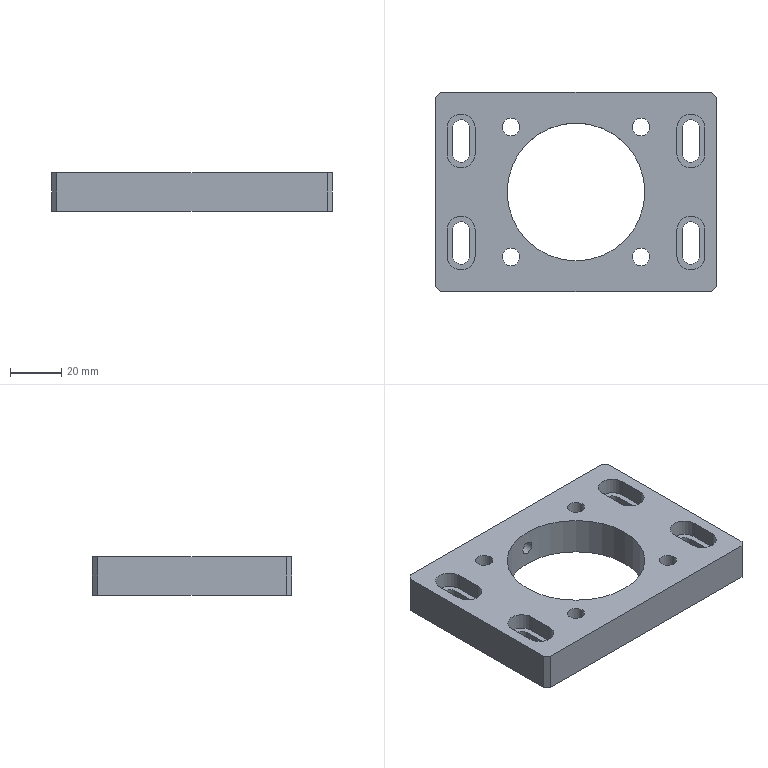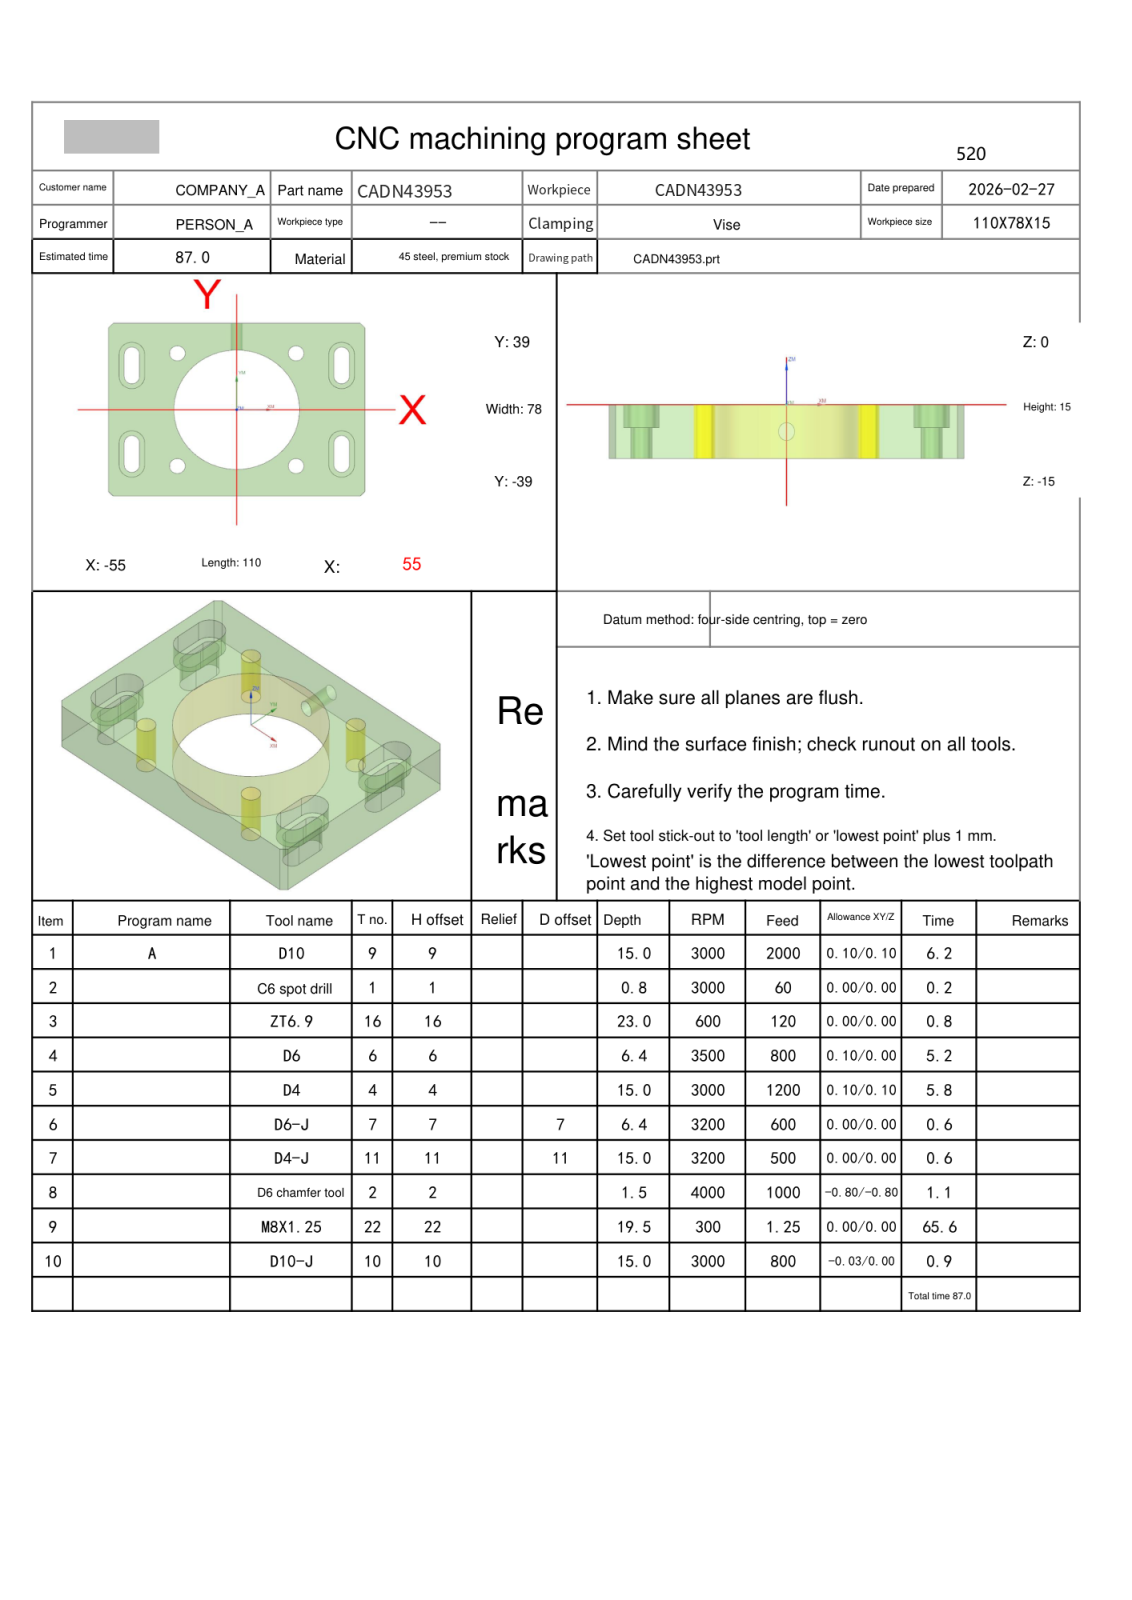NC program | NX | posted by the shop | part box 110 x 78 x 15 mm
Lines 2258 to 4088 of 4469, first 1188 of 1831 lines:
N5 T04 M06
(D4  D=4. R=0. H=04 ce=0.10 di=0.10)
G00 G90 G54 X-46.2 Y-20. M03 S3000
G43 H04 Z50.
M08
Z-5.9
G01 Y-25. Z-5.927 F1200.
G03 X-45. Y-26.2 Z-5.937 I1.2 J0.0
X-43.8 Y-25. Z-5.948 I0.0 J1.2
G01 Y-15. Z-6.002
G03 X-45. Y-13.8 Z-6.012 I-1.2 J0.0
X-46.2 Y-15. Z-6.022 I0.0 J-1.2
G01 Y-25. Z-6.076
G03 X-45. Y-26.2 Z-6.086 I1.2 J0.0
X-43.8 Y-25. Z-6.097 I0.0 J1.2
G01 Y-15. Z-6.151
G03 X-45. Y-13.8 Z-6.161 I-1.2 J0.0
X-46.2 Y-15. Z-6.171 I0.0 J-1.2
G01 Y-25. Z-6.225
G03 X-45. Y-26.2 Z-6.236 I1.2 J0.0
X-43.8 Y-25. Z-6.246 I0.0 J1.2
G01 Y-15. Z-6.3
G03 X-45. Y-13.8 Z-6.31 I-1.2 J0.0
X-46.2 Y-15. Z-6.32 I0.0 J-1.2
G01 Y-25. Z-6.375
G03 X-45. Y-26.2 Z-6.385 I1.2 J0.0
X-43.8 Y-25. Z-6.395 I0.0 J1.2
G01 Y-15. Z-6.449
G03 X-45. Y-13.8 Z-6.459 I-1.2 J0.0
X-46.2 Y-15. Z-6.47 I0.0 J-1.2
G01 Y-25. Z-6.524
G03 X-45. Y-26.2 Z-6.534 I1.2 J0.0
X-43.8 Y-25. Z-6.544 I0.0 J1.2
G01 Y-15. Z-6.598
G03 X-45. Y-13.8 Z-6.609 I-1.2 J0.0
X-46.2 Y-15. Z-6.619 I0.0 J-1.2
G01 Y-25. Z-6.673
G03 X-45. Y-26.2 Z-6.683 I1.2 J0.0
X-43.8 Y-25. Z-6.693 I0.0 J1.2
G01 Y-15. Z-6.748
G03 X-45. Y-13.8 Z-6.758 I-1.2 J0.0
X-46.2 Y-15. Z-6.768 I0.0 J-1.2
G01 Y-25. Z-6.822
G03 X-45. Y-26.2 Z-6.832 I1.2 J0.0
X-43.8 Y-25. Z-6.843 I0.0 J1.2
G01 Y-15. Z-6.897
G03 X-45. Y-13.8 Z-6.907 I-1.2 J0.0
X-46.2 Y-15. Z-6.917 I0.0 J-1.2
G01 Y-25. Z-6.971
G03 X-45. Y-26.2 Z-6.982 I1.2 J0.0
X-43.8 Y-25. Z-6.992 I0.0 J1.2
G01 Y-15. Z-7.046
G03 X-45. Y-13.8 Z-7.056 I-1.2 J0.0
X-46.2 Y-15. Z-7.066 I0.0 J-1.2
G01 Y-25. Z-7.121
G03 X-45. Y-26.2 Z-7.131 I1.2 J0.0
X-43.8 Y-25. Z-7.141 I0.0 J1.2
G01 Y-15. Z-7.195
G03 X-45. Y-13.8 Z-7.205 I-1.2 J0.0
X-46.2 Y-15. Z-7.216 I0.0 J-1.2
G01 Y-25. Z-7.27
G03 X-45. Y-26.2 Z-7.28 I1.2 J0.0
X-43.8 Y-25. Z-7.29 I0.0 J1.2
G01 Y-15. Z-7.344
G03 X-45. Y-13.8 Z-7.355 I-1.2 J0.0
X-46.2 Y-15. Z-7.365 I0.0 J-1.2
G01 Y-25. Z-7.419
G03 X-45. Y-26.2 Z-7.429 I1.2 J0.0
X-43.8 Y-25. Z-7.439 I0.0 J1.2
G01 Y-15. Z-7.493
G03 X-45. Y-13.8 Z-7.504 I-1.2 J0.0
X-46.2 Y-15. Z-7.514 I0.0 J-1.2
G01 Y-25. Z-7.568
G03 X-45. Y-26.2 Z-7.578 I1.2 J0.0
X-43.8 Y-25. Z-7.588 I0.0 J1.2
G01 Y-15. Z-7.643
G03 X-45. Y-13.8 Z-7.653 I-1.2 J0.0
X-46.2 Y-15. Z-7.663 I0.0 J-1.2
G01 Y-25. Z-7.717
G03 X-45. Y-26.2 Z-7.727 I1.2 J0.0
X-43.8 Y-25. Z-7.738 I0.0 J1.2
G01 Y-15. Z-7.792
G03 X-45. Y-13.8 Z-7.802 I-1.2 J0.0
X-46.2 Y-15. Z-7.812 I0.0 J-1.2
G01 Y-25. Z-7.866
G03 X-45. Y-26.2 Z-7.877 I1.2 J0.0
X-43.8 Y-25. Z-7.887 I0.0 J1.2
G01 Y-15. Z-7.941
G03 X-45. Y-13.8 Z-7.951 I-1.2 J0.0
X-46.2 Y-15. Z-7.961 I0.0 J-1.2
G01 Y-25. Z-8.016
G03 X-45. Y-26.2 Z-8.026 I1.2 J0.0
X-43.8 Y-25. Z-8.036 I0.0 J1.2
G01 Y-15. Z-8.09
G03 X-45. Y-13.8 Z-8.1 I-1.2 J0.0
X-46.2 Y-15. Z-8.111 I0.0 J-1.2
G01 Y-25. Z-8.165
G03 X-45. Y-26.2 Z-8.175 I1.2 J0.0
X-43.8 Y-25. Z-8.185 I0.0 J1.2
G01 Y-15. Z-8.239
G03 X-45. Y-13.8 Z-8.25 I-1.2 J0.0
X-46.2 Y-15. Z-8.26 I0.0 J-1.2
G01 Y-25. Z-8.314
G03 X-45. Y-26.2 Z-8.324 I1.2 J0.0
X-43.8 Y-25. Z-8.334 I0.0 J1.2
G01 Y-15. Z-8.389
G03 X-45. Y-13.8 Z-8.399 I-1.2 J0.0
X-46.2 Y-15. Z-8.409 I0.0 J-1.2
G01 Y-25. Z-8.463
G03 X-45. Y-26.2 Z-8.473 I1.2 J0.0
X-43.8 Y-25. Z-8.484 I0.0 J1.2
G01 Y-15. Z-8.538
G03 X-45. Y-13.8 Z-8.548 I-1.2 J0.0
X-46.2 Y-15. Z-8.558 I0.0 J-1.2
G01 Y-25. Z-8.612
G03 X-45. Y-26.2 Z-8.623 I1.2 J0.0
X-43.8 Y-25. Z-8.633 I0.0 J1.2
G01 Y-15. Z-8.687
G03 X-45. Y-13.8 Z-8.697 I-1.2 J0.0
X-46.2 Y-15. Z-8.707 I0.0 J-1.2
G01 Y-25. Z-8.762
G03 X-45. Y-26.2 Z-8.772 I1.2 J0.0
X-43.8 Y-25. Z-8.782 I0.0 J1.2
G01 Y-15. Z-8.836
G03 X-45. Y-13.8 Z-8.846 I-1.2 J0.0
X-46.2 Y-15. Z-8.857 I0.0 J-1.2
G01 Y-25. Z-8.911
G03 X-45. Y-26.2 Z-8.921 I1.2 J0.0
X-43.8 Y-25. Z-8.931 I0.0 J1.2
G01 Y-15. Z-8.985
G03 X-45. Y-13.8 Z-8.995 I-1.2 J0.0
X-46.2 Y-15. Z-9.006 I0.0 J-1.2
G01 Y-25. Z-9.06
G03 X-45. Y-26.2 Z-9.07 I1.2 J0.0
X-43.8 Y-25. Z-9.08 I0.0 J1.2
G01 Y-15. Z-9.134
G03 X-45. Y-13.8 Z-9.145 I-1.2 J0.0
X-46.2 Y-15. Z-9.155 I0.0 J-1.2
G01 Y-25. Z-9.209
G03 X-45. Y-26.2 Z-9.219 I1.2 J0.0
X-43.8 Y-25. Z-9.229 I0.0 J1.2
G01 Y-15. Z-9.284
G03 X-45. Y-13.8 Z-9.294 I-1.2 J0.0
X-46.2 Y-15. Z-9.304 I0.0 J-1.2
G01 Y-25. Z-9.358
G03 X-45. Y-26.2 Z-9.368 I1.2 J0.0
X-43.8 Y-25. Z-9.379 I0.0 J1.2
G01 Y-15. Z-9.433
G03 X-45. Y-13.8 Z-9.443 I-1.2 J0.0
X-46.2 Y-15. Z-9.453 I0.0 J-1.2
G01 Y-25. Z-9.507
G03 X-45. Y-26.2 Z-9.518 I1.2 J0.0
X-43.8 Y-25. Z-9.528 I0.0 J1.2
G01 Y-15. Z-9.582
G03 X-45. Y-13.8 Z-9.592 I-1.2 J0.0
X-46.2 Y-15. Z-9.602 I0.0 J-1.2
G01 Y-25. Z-9.657
G03 X-45. Y-26.2 Z-9.667 I1.2 J0.0
X-43.8 Y-25. Z-9.677 I0.0 J1.2
G01 Y-15. Z-9.731
G03 X-45. Y-13.8 Z-9.741 I-1.2 J0.0
X-46.2 Y-15. Z-9.752 I0.0 J-1.2
G01 Y-25. Z-9.806
G03 X-45. Y-26.2 Z-9.816 I1.2 J0.0
X-43.8 Y-25. Z-9.826 I0.0 J1.2
G01 Y-15. Z-9.88
G03 X-45. Y-13.8 Z-9.891 I-1.2 J0.0
X-46.2 Y-15. Z-9.901 I0.0 J-1.2
G01 Y-25. Z-9.955
G03 X-45. Y-26.2 Z-9.965 I1.2 J0.0
X-43.8 Y-25. Z-9.975 I0.0 J1.2
G01 Y-15. Z-10.03
G03 X-45. Y-13.8 Z-10.04 I-1.2 J0.0
X-46.2 Y-15. Z-10.05 I0.0 J-1.2
G01 Y-25. Z-10.104
G03 X-45. Y-26.2 Z-10.114 I1.2 J0.0
X-43.8 Y-25. Z-10.125 I0.0 J1.2
G01 Y-15. Z-10.179
G03 X-45. Y-13.8 Z-10.189 I-1.2 J0.0
X-46.2 Y-15. Z-10.199 I0.0 J-1.2
G01 Y-25. Z-10.253
G03 X-45. Y-26.2 Z-10.264 I1.2 J0.0
X-43.8 Y-25. Z-10.274 I0.0 J1.2
G01 Y-15. Z-10.328
G03 X-45. Y-13.8 Z-10.338 I-1.2 J0.0
X-46.2 Y-15. Z-10.348 I0.0 J-1.2
G01 Y-25. Z-10.402
G03 X-45. Y-26.2 Z-10.413 I1.2 J0.0
X-43.8 Y-25. Z-10.423 I0.0 J1.2
G01 Y-15. Z-10.477
G03 X-45. Y-13.8 Z-10.487 I-1.2 J0.0
X-46.2 Y-15. Z-10.498 I0.0 J-1.2
G01 Y-25. Z-10.552
G03 X-45. Y-26.2 Z-10.562 I1.2 J0.0
X-43.8 Y-25. Z-10.572 I0.0 J1.2
G01 Y-15. Z-10.626
G03 X-45. Y-13.8 Z-10.636 I-1.2 J0.0
X-46.2 Y-15. Z-10.647 I0.0 J-1.2
G01 Y-25. Z-10.701
G03 X-45. Y-26.2 Z-10.711 I1.2 J0.0
X-43.8 Y-25. Z-10.721 I0.0 J1.2
G01 Y-15. Z-10.775
G03 X-45. Y-13.8 Z-10.786 I-1.2 J0.0
X-46.2 Y-15. Z-10.796 I0.0 J-1.2
G01 Y-25. Z-10.85
G03 X-45. Y-26.2 Z-10.86 I1.2 J0.0
X-43.8 Y-25. Z-10.87 I0.0 J1.2
G01 Y-15. Z-10.925
G03 X-45. Y-13.8 Z-10.935 I-1.2 J0.0
X-46.2 Y-15. Z-10.945 I0.0 J-1.2
G01 Y-25. Z-10.999
G03 X-45. Y-26.2 Z-11.009 I1.2 J0.0
X-43.8 Y-25. Z-11.02 I0.0 J1.2
G01 Y-15. Z-11.074
G03 X-45. Y-13.8 Z-11.084 I-1.2 J0.0
X-46.2 Y-15. Z-11.094 I0.0 J-1.2
G01 Y-25. Z-11.148
G03 X-45. Y-26.2 Z-11.159 I1.2 J0.0
X-43.8 Y-25. Z-11.169 I0.0 J1.2
G01 Y-15. Z-11.223
G03 X-45. Y-13.8 Z-11.233 I-1.2 J0.0
X-46.2 Y-15. Z-11.243 I0.0 J-1.2
G01 Y-25. Z-11.298
G03 X-45. Y-26.2 Z-11.308 I1.2 J0.0
X-43.8 Y-25. Z-11.318 I0.0 J1.2
G01 Y-15. Z-11.372
G03 X-45. Y-13.8 Z-11.382 I-1.2 J0.0
X-46.2 Y-15. Z-11.393 I0.0 J-1.2
G01 Y-25. Z-11.447
G03 X-45. Y-26.2 Z-11.457 I1.2 J0.0
X-43.8 Y-25. Z-11.467 I0.0 J1.2
G01 Y-15. Z-11.521
G03 X-45. Y-13.8 Z-11.532 I-1.2 J0.0
X-46.2 Y-15. Z-11.542 I0.0 J-1.2
G01 Y-25. Z-11.596
G03 X-45. Y-26.2 Z-11.606 I1.2 J0.0
X-43.8 Y-25. Z-11.616 I0.0 J1.2
G01 Y-15. Z-11.671
G03 X-45. Y-13.8 Z-11.681 I-1.2 J0.0
X-46.2 Y-15. Z-11.691 I0.0 J-1.2
G01 Y-25. Z-11.745
G03 X-45. Y-26.2 Z-11.755 I1.2 J0.0
X-43.8 Y-25. Z-11.766 I0.0 J1.2
G01 Y-15. Z-11.82
G03 X-45. Y-13.8 Z-11.83 I-1.2 J0.0
X-46.2 Y-15. Z-11.84 I0.0 J-1.2
G01 Y-25. Z-11.894
G03 X-45. Y-26.2 Z-11.905 I1.2 J0.0
X-43.8 Y-25. Z-11.915 I0.0 J1.2
G01 Y-15. Z-11.969
G03 X-45. Y-13.8 Z-11.979 I-1.2 J0.0
X-46.2 Y-15. Z-11.989 I0.0 J-1.2
G01 Y-25. Z-12.043
G03 X-45. Y-26.2 Z-12.054 I1.2 J0.0
X-43.8 Y-25. Z-12.064 I0.0 J1.2
G01 Y-15. Z-12.118
G03 X-45. Y-13.8 Z-12.128 I-1.2 J0.0
X-46.2 Y-15. Z-12.138 I0.0 J-1.2
G01 Y-25. Z-12.193
G03 X-45. Y-26.2 Z-12.203 I1.2 J0.0
X-43.8 Y-25. Z-12.213 I0.0 J1.2
G01 Y-15. Z-12.267
G03 X-45. Y-13.8 Z-12.277 I-1.2 J0.0
X-46.2 Y-15. Z-12.288 I0.0 J-1.2
G01 Y-25. Z-12.342
G03 X-45. Y-26.2 Z-12.352 I1.2 J0.0
X-43.8 Y-25. Z-12.362 I0.0 J1.2
G01 Y-15. Z-12.416
G03 X-45. Y-13.8 Z-12.427 I-1.2 J0.0
X-46.2 Y-15. Z-12.437 I0.0 J-1.2
G01 Y-25. Z-12.491
G03 X-45. Y-26.2 Z-12.501 I1.2 J0.0
X-43.8 Y-25. Z-12.511 I0.0 J1.2
G01 Y-15. Z-12.566
G03 X-45. Y-13.8 Z-12.576 I-1.2 J0.0
X-46.2 Y-15. Z-12.586 I0.0 J-1.2
G01 Y-25. Z-12.64
G03 X-45. Y-26.2 Z-12.65 I1.2 J0.0
X-43.8 Y-25. Z-12.661 I0.0 J1.2
G01 Y-15. Z-12.715
G03 X-45. Y-13.8 Z-12.725 I-1.2 J0.0
X-46.2 Y-15. Z-12.735 I0.0 J-1.2
G01 Y-25. Z-12.789
G03 X-45. Y-26.2 Z-12.8 I1.2 J0.0
X-43.8 Y-25. Z-12.81 I0.0 J1.2
G01 Y-15. Z-12.864
G03 X-45. Y-13.8 Z-12.874 I-1.2 J0.0
X-46.2 Y-15. Z-12.884 I0.0 J-1.2
G01 Y-25. Z-12.939
G03 X-45. Y-26.2 Z-12.949 I1.2 J0.0
X-43.8 Y-25. Z-12.959 I0.0 J1.2
G01 Y-15. Z-13.013
G03 X-45. Y-13.8 Z-13.023 I-1.2 J0.0
X-46.2 Y-15. Z-13.034 I0.0 J-1.2
G01 Y-25. Z-13.088
G03 X-45. Y-26.2 Z-13.098 I1.2 J0.0
X-43.8 Y-25. Z-13.108 I0.0 J1.2
G01 Y-15. Z-13.162
G03 X-45. Y-13.8 Z-13.173 I-1.2 J0.0
X-46.2 Y-15. Z-13.183 I0.0 J-1.2
G01 Y-25. Z-13.237
G03 X-45. Y-26.2 Z-13.247 I1.2 J0.0
X-43.8 Y-25. Z-13.257 I0.0 J1.2
G01 Y-15. Z-13.312
G03 X-45. Y-13.8 Z-13.322 I-1.2 J0.0
X-46.2 Y-15. Z-13.332 I0.0 J-1.2
G01 Y-25. Z-13.386
G03 X-45. Y-26.2 Z-13.396 I1.2 J0.0
X-43.8 Y-25. Z-13.407 I0.0 J1.2
G01 Y-15. Z-13.461
G03 X-45. Y-13.8 Z-13.471 I-1.2 J0.0
X-46.2 Y-15. Z-13.481 I0.0 J-1.2
G01 Y-25. Z-13.535
G03 X-45. Y-26.2 Z-13.545 I1.2 J0.0
X-43.8 Y-25. Z-13.556 I0.0 J1.2
G01 Y-15. Z-13.61
G03 X-45. Y-13.8 Z-13.62 I-1.2 J0.0
X-46.2 Y-15. Z-13.63 I0.0 J-1.2
G01 Y-25. Z-13.684
G03 X-45. Y-26.2 Z-13.695 I1.2 J0.0
X-43.8 Y-25. Z-13.705 I0.0 J1.2
G01 Y-15. Z-13.759
G03 X-45. Y-13.8 Z-13.769 I-1.2 J0.0
X-46.2 Y-15. Z-13.779 I0.0 J-1.2
G01 Y-25. Z-13.834
G03 X-45. Y-26.2 Z-13.844 I1.2 J0.0
X-43.8 Y-25. Z-13.854 I0.0 J1.2
G01 Y-15. Z-13.908
G03 X-45. Y-13.8 Z-13.918 I-1.2 J0.0
X-46.2 Y-15. Z-13.929 I0.0 J-1.2
G01 Y-25. Z-13.983
G03 X-45. Y-26.2 Z-13.993 I1.2 J0.0
X-43.8 Y-25. Z-14.003 I0.0 J1.2
G01 Y-15. Z-14.057
G03 X-45. Y-13.8 Z-14.068 I-1.2 J0.0
X-46.2 Y-15. Z-14.078 I0.0 J-1.2
G01 Y-25. Z-14.132
G03 X-45. Y-26.2 Z-14.142 I1.2 J0.0
X-43.8 Y-25. Z-14.152 I0.0 J1.2
G01 Y-15. Z-14.207
G03 X-45. Y-13.8 Z-14.217 I-1.2 J0.0
X-46.2 Y-15. Z-14.227 I0.0 J-1.2
G01 Y-25. Z-14.281
G03 X-45. Y-26.2 Z-14.291 I1.2 J0.0
X-43.8 Y-25. Z-14.302 I0.0 J1.2
G01 Y-15. Z-14.356
G03 X-45. Y-13.8 Z-14.366 I-1.2 J0.0
X-46.2 Y-15. Z-14.376 I0.0 J-1.2
G01 Y-25. Z-14.43
G03 X-45. Y-26.2 Z-14.441 I1.2 J0.0
X-43.8 Y-25. Z-14.451 I0.0 J1.2
G01 Y-15. Z-14.505
G03 X-45. Y-13.8 Z-14.515 I-1.2 J0.0
X-46.2 Y-15. Z-14.525 I0.0 J-1.2
G01 Y-25. Z-14.58
G03 X-45. Y-26.2 Z-14.59 I1.2 J0.0
X-43.8 Y-25. Z-14.6 I0.0 J1.2
G01 Y-15. Z-14.654
G03 X-45. Y-13.8 Z-14.664 I-1.2 J0.0
X-46.2 Y-15. Z-14.675 I0.0 J-1.2
G01 Y-25. Z-14.729
G03 X-45. Y-26.2 Z-14.739 I1.2 J0.0
X-43.8 Y-25. Z-14.749 I0.0 J1.2
G01 Y-15. Z-14.803
G03 X-45. Y-13.8 Z-14.814 I-1.2 J0.0
X-46.2 Y-15. Z-14.824 I0.0 J-1.2
G01 Y-25. Z-14.878
G03 X-45. Y-26.2 Z-14.888 I1.2 J0.0
X-43.8 Y-25. Z-14.898 I0.0 J1.2
G01 Y-15. Z-14.952
G03 X-45. Y-13.8 Z-14.963 I-1.2 J0.0
X-46.2 Y-15. Z-14.973 I0.0 J-1.2
G01 Y-20. Z-15.
Y-25.
G03 X-45. Y-26.2 I1.2 J0.0
X-43.8 Y-25. I0.0 J1.2
G01 Y-15.
G03 X-45. Y-13.8 I-1.2 J0.0
X-46.2 Y-15. I0.0 J-1.2
G01 Y-20.
Y-20.5
Z-14.
G00 Z50.
Y20.
Z-5.9
G01 Y15. Z-5.927
G03 X-45. Y13.8 Z-5.937 I1.2 J0.0
X-43.8 Y15. Z-5.948 I0.0 J1.2
G01 Y25. Z-6.002
G03 X-45. Y26.2 Z-6.012 I-1.2 J0.0
X-46.2 Y25. Z-6.022 I0.0 J-1.2
G01 Y15. Z-6.076
G03 X-45. Y13.8 Z-6.086 I1.2 J0.0
X-43.8 Y15. Z-6.097 I0.0 J1.2
G01 Y25. Z-6.151
G03 X-45. Y26.2 Z-6.161 I-1.2 J0.0
X-46.2 Y25. Z-6.171 I0.0 J-1.2
G01 Y15. Z-6.225
G03 X-45. Y13.8 Z-6.236 I1.2 J0.0
X-43.8 Y15. Z-6.246 I0.0 J1.2
G01 Y25. Z-6.3
G03 X-45. Y26.2 Z-6.31 I-1.2 J0.0
X-46.2 Y25. Z-6.32 I0.0 J-1.2
G01 Y15. Z-6.375
G03 X-45. Y13.8 Z-6.385 I1.2 J0.0
X-43.8 Y15. Z-6.395 I0.0 J1.2
G01 Y25. Z-6.449
G03 X-45. Y26.2 Z-6.459 I-1.2 J0.0
X-46.2 Y25. Z-6.47 I0.0 J-1.2
G01 Y15. Z-6.524
G03 X-45. Y13.8 Z-6.534 I1.2 J0.0
X-43.8 Y15. Z-6.544 I0.0 J1.2
G01 Y25. Z-6.598
G03 X-45. Y26.2 Z-6.609 I-1.2 J0.0
X-46.2 Y25. Z-6.619 I0.0 J-1.2
G01 Y15. Z-6.673
G03 X-45. Y13.8 Z-6.683 I1.2 J0.0
X-43.8 Y15. Z-6.693 I0.0 J1.2
G01 Y25. Z-6.748
G03 X-45. Y26.2 Z-6.758 I-1.2 J0.0
X-46.2 Y25. Z-6.768 I0.0 J-1.2
G01 Y15. Z-6.822
G03 X-45. Y13.8 Z-6.832 I1.2 J0.0
X-43.8 Y15. Z-6.843 I0.0 J1.2
G01 Y25. Z-6.897
G03 X-45. Y26.2 Z-6.907 I-1.2 J0.0
X-46.2 Y25. Z-6.917 I0.0 J-1.2
G01 Y15. Z-6.971
G03 X-45. Y13.8 Z-6.982 I1.2 J0.0
X-43.8 Y15. Z-6.992 I0.0 J1.2
G01 Y25. Z-7.046
G03 X-45. Y26.2 Z-7.056 I-1.2 J0.0
X-46.2 Y25. Z-7.066 I0.0 J-1.2
G01 Y15. Z-7.121
G03 X-45. Y13.8 Z-7.131 I1.2 J0.0
X-43.8 Y15. Z-7.141 I0.0 J1.2
G01 Y25. Z-7.195
G03 X-45. Y26.2 Z-7.205 I-1.2 J0.0
X-46.2 Y25. Z-7.216 I0.0 J-1.2
G01 Y15. Z-7.27
G03 X-45. Y13.8 Z-7.28 I1.2 J0.0
X-43.8 Y15. Z-7.29 I0.0 J1.2
G01 Y25. Z-7.344
G03 X-45. Y26.2 Z-7.355 I-1.2 J0.0
X-46.2 Y25. Z-7.365 I0.0 J-1.2
G01 Y15. Z-7.419
G03 X-45. Y13.8 Z-7.429 I1.2 J0.0
X-43.8 Y15. Z-7.439 I0.0 J1.2
G01 Y25. Z-7.493
G03 X-45. Y26.2 Z-7.504 I-1.2 J0.0
X-46.2 Y25. Z-7.514 I0.0 J-1.2
G01 Y15. Z-7.568
G03 X-45. Y13.8 Z-7.578 I1.2 J0.0
X-43.8 Y15. Z-7.588 I0.0 J1.2
G01 Y25. Z-7.643
G03 X-45. Y26.2 Z-7.653 I-1.2 J0.0
X-46.2 Y25. Z-7.663 I0.0 J-1.2
G01 Y15. Z-7.717
G03 X-45. Y13.8 Z-7.727 I1.2 J0.0
X-43.8 Y15. Z-7.738 I0.0 J1.2
G01 Y25. Z-7.792
G03 X-45. Y26.2 Z-7.802 I-1.2 J0.0
X-46.2 Y25. Z-7.812 I0.0 J-1.2
G01 Y15. Z-7.866
G03 X-45. Y13.8 Z-7.877 I1.2 J0.0
X-43.8 Y15. Z-7.887 I0.0 J1.2
G01 Y25. Z-7.941
G03 X-45. Y26.2 Z-7.951 I-1.2 J0.0
X-46.2 Y25. Z-7.961 I0.0 J-1.2
G01 Y15. Z-8.016
G03 X-45. Y13.8 Z-8.026 I1.2 J0.0
X-43.8 Y15. Z-8.036 I0.0 J1.2
G01 Y25. Z-8.09
G03 X-45. Y26.2 Z-8.1 I-1.2 J0.0
X-46.2 Y25. Z-8.111 I0.0 J-1.2
G01 Y15. Z-8.165
G03 X-45. Y13.8 Z-8.175 I1.2 J0.0
X-43.8 Y15. Z-8.185 I0.0 J1.2
G01 Y25. Z-8.239
G03 X-45. Y26.2 Z-8.25 I-1.2 J0.0
X-46.2 Y25. Z-8.26 I0.0 J-1.2
G01 Y15. Z-8.314
G03 X-45. Y13.8 Z-8.324 I1.2 J0.0
X-43.8 Y15. Z-8.334 I0.0 J1.2
G01 Y25. Z-8.389
G03 X-45. Y26.2 Z-8.399 I-1.2 J0.0
X-46.2 Y25. Z-8.409 I0.0 J-1.2
G01 Y15. Z-8.463
G03 X-45. Y13.8 Z-8.473 I1.2 J0.0
X-43.8 Y15. Z-8.484 I0.0 J1.2
G01 Y25. Z-8.538
G03 X-45. Y26.2 Z-8.548 I-1.2 J0.0
X-46.2 Y25. Z-8.558 I0.0 J-1.2
G01 Y15. Z-8.612
G03 X-45. Y13.8 Z-8.623 I1.2 J0.0
X-43.8 Y15. Z-8.633 I0.0 J1.2
G01 Y25. Z-8.687
G03 X-45. Y26.2 Z-8.697 I-1.2 J0.0
X-46.2 Y25. Z-8.707 I0.0 J-1.2
G01 Y15. Z-8.762
G03 X-45. Y13.8 Z-8.772 I1.2 J0.0
X-43.8 Y15. Z-8.782 I0.0 J1.2
G01 Y25. Z-8.836
G03 X-45. Y26.2 Z-8.846 I-1.2 J0.0
X-46.2 Y25. Z-8.857 I0.0 J-1.2
G01 Y15. Z-8.911
G03 X-45. Y13.8 Z-8.921 I1.2 J0.0
X-43.8 Y15. Z-8.931 I0.0 J1.2
G01 Y25. Z-8.985
G03 X-45. Y26.2 Z-8.995 I-1.2 J0.0
X-46.2 Y25. Z-9.006 I0.0 J-1.2
G01 Y15. Z-9.06
G03 X-45. Y13.8 Z-9.07 I1.2 J0.0
X-43.8 Y15. Z-9.08 I0.0 J1.2
G01 Y25. Z-9.134
G03 X-45. Y26.2 Z-9.145 I-1.2 J0.0
X-46.2 Y25. Z-9.155 I0.0 J-1.2
G01 Y15. Z-9.209
G03 X-45. Y13.8 Z-9.219 I1.2 J0.0
X-43.8 Y15. Z-9.229 I0.0 J1.2
G01 Y25. Z-9.284
G03 X-45. Y26.2 Z-9.294 I-1.2 J0.0
X-46.2 Y25. Z-9.304 I0.0 J-1.2
G01 Y15. Z-9.358
G03 X-45. Y13.8 Z-9.368 I1.2 J0.0
X-43.8 Y15. Z-9.379 I0.0 J1.2
G01 Y25. Z-9.433
G03 X-45. Y26.2 Z-9.443 I-1.2 J0.0
X-46.2 Y25. Z-9.453 I0.0 J-1.2
G01 Y15. Z-9.507
G03 X-45. Y13.8 Z-9.518 I1.2 J0.0
X-43.8 Y15. Z-9.528 I0.0 J1.2
G01 Y25. Z-9.582
G03 X-45. Y26.2 Z-9.592 I-1.2 J0.0
X-46.2 Y25. Z-9.602 I0.0 J-1.2
G01 Y15. Z-9.657
G03 X-45. Y13.8 Z-9.667 I1.2 J0.0
X-43.8 Y15. Z-9.677 I0.0 J1.2
G01 Y25. Z-9.731
G03 X-45. Y26.2 Z-9.741 I-1.2 J0.0
X-46.2 Y25. Z-9.752 I0.0 J-1.2
G01 Y15. Z-9.806
G03 X-45. Y13.8 Z-9.816 I1.2 J0.0
X-43.8 Y15. Z-9.826 I0.0 J1.2
G01 Y25. Z-9.88
G03 X-45. Y26.2 Z-9.891 I-1.2 J0.0
X-46.2 Y25. Z-9.901 I0.0 J-1.2
G01 Y15. Z-9.955
G03 X-45. Y13.8 Z-9.965 I1.2 J0.0
X-43.8 Y15. Z-9.975 I0.0 J1.2
G01 Y25. Z-10.03
G03 X-45. Y26.2 Z-10.04 I-1.2 J0.0
X-46.2 Y25. Z-10.05 I0.0 J-1.2
G01 Y15. Z-10.104
G03 X-45. Y13.8 Z-10.114 I1.2 J0.0
X-43.8 Y15. Z-10.125 I0.0 J1.2
G01 Y25. Z-10.179
G03 X-45. Y26.2 Z-10.189 I-1.2 J0.0
X-46.2 Y25. Z-10.199 I0.0 J-1.2
G01 Y15. Z-10.253
G03 X-45. Y13.8 Z-10.264 I1.2 J0.0
X-43.8 Y15. Z-10.274 I0.0 J1.2
G01 Y25. Z-10.328
G03 X-45. Y26.2 Z-10.338 I-1.2 J0.0
X-46.2 Y25. Z-10.348 I0.0 J-1.2
G01 Y15. Z-10.402
G03 X-45. Y13.8 Z-10.413 I1.2 J0.0
X-43.8 Y15. Z-10.423 I0.0 J1.2
G01 Y25. Z-10.477
G03 X-45. Y26.2 Z-10.487 I-1.2 J0.0
X-46.2 Y25. Z-10.498 I0.0 J-1.2
G01 Y15. Z-10.552
G03 X-45. Y13.8 Z-10.562 I1.2 J0.0
X-43.8 Y15. Z-10.572 I0.0 J1.2
G01 Y25. Z-10.626
G03 X-45. Y26.2 Z-10.636 I-1.2 J0.0
X-46.2 Y25. Z-10.647 I0.0 J-1.2
G01 Y15. Z-10.701
G03 X-45. Y13.8 Z-10.711 I1.2 J0.0
X-43.8 Y15. Z-10.721 I0.0 J1.2
G01 Y25. Z-10.775
G03 X-45. Y26.2 Z-10.786 I-1.2 J0.0
X-46.2 Y25. Z-10.796 I0.0 J-1.2
G01 Y15. Z-10.85
G03 X-45. Y13.8 Z-10.86 I1.2 J0.0
X-43.8 Y15. Z-10.87 I0.0 J1.2
G01 Y25. Z-10.925
G03 X-45. Y26.2 Z-10.935 I-1.2 J0.0
X-46.2 Y25. Z-10.945 I0.0 J-1.2
G01 Y15. Z-10.999
G03 X-45. Y13.8 Z-11.009 I1.2 J0.0
X-43.8 Y15. Z-11.02 I0.0 J1.2
G01 Y25. Z-11.074
G03 X-45. Y26.2 Z-11.084 I-1.2 J0.0
X-46.2 Y25. Z-11.094 I0.0 J-1.2
G01 Y15. Z-11.148
G03 X-45. Y13.8 Z-11.159 I1.2 J0.0
X-43.8 Y15. Z-11.169 I0.0 J1.2
G01 Y25. Z-11.223
G03 X-45. Y26.2 Z-11.233 I-1.2 J0.0
X-46.2 Y25. Z-11.243 I0.0 J-1.2
G01 Y15. Z-11.298
G03 X-45. Y13.8 Z-11.308 I1.2 J0.0
X-43.8 Y15. Z-11.318 I0.0 J1.2
G01 Y25. Z-11.372
G03 X-45. Y26.2 Z-11.382 I-1.2 J0.0
X-46.2 Y25. Z-11.393 I0.0 J-1.2
G01 Y15. Z-11.447
G03 X-45. Y13.8 Z-11.457 I1.2 J0.0
X-43.8 Y15. Z-11.467 I0.0 J1.2
G01 Y25. Z-11.521
G03 X-45. Y26.2 Z-11.532 I-1.2 J0.0
X-46.2 Y25. Z-11.542 I0.0 J-1.2
G01 Y15. Z-11.596
G03 X-45. Y13.8 Z-11.606 I1.2 J0.0
X-43.8 Y15. Z-11.616 I0.0 J1.2
G01 Y25. Z-11.671
G03 X-45. Y26.2 Z-11.681 I-1.2 J0.0
X-46.2 Y25. Z-11.691 I0.0 J-1.2
G01 Y15. Z-11.745
G03 X-45. Y13.8 Z-11.755 I1.2 J0.0
X-43.8 Y15. Z-11.766 I0.0 J1.2
G01 Y25. Z-11.82
G03 X-45. Y26.2 Z-11.83 I-1.2 J0.0
X-46.2 Y25. Z-11.84 I0.0 J-1.2
G01 Y15. Z-11.894
G03 X-45. Y13.8 Z-11.905 I1.2 J0.0
X-43.8 Y15. Z-11.915 I0.0 J1.2
G01 Y25. Z-11.969
G03 X-45. Y26.2 Z-11.979 I-1.2 J0.0
X-46.2 Y25. Z-11.989 I0.0 J-1.2
G01 Y15. Z-12.043
G03 X-45. Y13.8 Z-12.054 I1.2 J0.0
X-43.8 Y15. Z-12.064 I0.0 J1.2
G01 Y25. Z-12.118
G03 X-45. Y26.2 Z-12.128 I-1.2 J0.0
X-46.2 Y25. Z-12.138 I0.0 J-1.2
G01 Y15. Z-12.193
G03 X-45. Y13.8 Z-12.203 I1.2 J0.0
X-43.8 Y15. Z-12.213 I0.0 J1.2
G01 Y25. Z-12.267
G03 X-45. Y26.2 Z-12.277 I-1.2 J0.0
X-46.2 Y25. Z-12.288 I0.0 J-1.2
G01 Y15. Z-12.342
G03 X-45. Y13.8 Z-12.352 I1.2 J0.0
X-43.8 Y15. Z-12.362 I0.0 J1.2
G01 Y25. Z-12.416
G03 X-45. Y26.2 Z-12.427 I-1.2 J0.0
X-46.2 Y25. Z-12.437 I0.0 J-1.2
G01 Y15. Z-12.491
G03 X-45. Y13.8 Z-12.501 I1.2 J0.0
X-43.8 Y15. Z-12.511 I0.0 J1.2
G01 Y25. Z-12.566
G03 X-45. Y26.2 Z-12.576 I-1.2 J0.0
X-46.2 Y25. Z-12.586 I0.0 J-1.2
G01 Y15. Z-12.64
G03 X-45. Y13.8 Z-12.65 I1.2 J0.0
X-43.8 Y15. Z-12.661 I0.0 J1.2
G01 Y25. Z-12.715
G03 X-45. Y26.2 Z-12.725 I-1.2 J0.0
X-46.2 Y25. Z-12.735 I0.0 J-1.2
G01 Y15. Z-12.789
G03 X-45. Y13.8 Z-12.8 I1.2 J0.0
X-43.8 Y15. Z-12.81 I0.0 J1.2
G01 Y25. Z-12.864
G03 X-45. Y26.2 Z-12.874 I-1.2 J0.0
X-46.2 Y25. Z-12.884 I0.0 J-1.2
G01 Y15. Z-12.939
G03 X-45. Y13.8 Z-12.949 I1.2 J0.0
X-43.8 Y15. Z-12.959 I0.0 J1.2
G01 Y25. Z-13.013
G03 X-45. Y26.2 Z-13.023 I-1.2 J0.0
X-46.2 Y25. Z-13.034 I0.0 J-1.2
G01 Y15. Z-13.088
G03 X-45. Y13.8 Z-13.098 I1.2 J0.0
X-43.8 Y15. Z-13.108 I0.0 J1.2
G01 Y25. Z-13.162
G03 X-45. Y26.2 Z-13.173 I-1.2 J0.0
X-46.2 Y25. Z-13.183 I0.0 J-1.2
G01 Y15. Z-13.237
G03 X-45. Y13.8 Z-13.247 I1.2 J0.0
X-43.8 Y15. Z-13.257 I0.0 J1.2
G01 Y25. Z-13.312
G03 X-45. Y26.2 Z-13.322 I-1.2 J0.0
X-46.2 Y25. Z-13.332 I0.0 J-1.2
G01 Y15. Z-13.386
G03 X-45. Y13.8 Z-13.396 I1.2 J0.0
X-43.8 Y15. Z-13.407 I0.0 J1.2
G01 Y25. Z-13.461
G03 X-45. Y26.2 Z-13.471 I-1.2 J0.0
X-46.2 Y25. Z-13.481 I0.0 J-1.2
G01 Y15. Z-13.535
G03 X-45. Y13.8 Z-13.545 I1.2 J0.0
X-43.8 Y15. Z-13.556 I0.0 J1.2
G01 Y25. Z-13.61
G03 X-45. Y26.2 Z-13.62 I-1.2 J0.0
X-46.2 Y25. Z-13.63 I0.0 J-1.2
G01 Y15. Z-13.684
G03 X-45. Y13.8 Z-13.695 I1.2 J0.0
X-43.8 Y15. Z-13.705 I0.0 J1.2
G01 Y25. Z-13.759
G03 X-45. Y26.2 Z-13.769 I-1.2 J0.0
X-46.2 Y25. Z-13.779 I0.0 J-1.2
G01 Y15. Z-13.834
G03 X-45. Y13.8 Z-13.844 I1.2 J0.0
X-43.8 Y15. Z-13.854 I0.0 J1.2
G01 Y25. Z-13.908
G03 X-45. Y26.2 Z-13.918 I-1.2 J0.0
X-46.2 Y25. Z-13.929 I0.0 J-1.2
G01 Y15. Z-13.983
G03 X-45. Y13.8 Z-13.993 I1.2 J0.0
X-43.8 Y15. Z-14.003 I0.0 J1.2
G01 Y25. Z-14.057
G03 X-45. Y26.2 Z-14.068 I-1.2 J0.0
X-46.2 Y25. Z-14.078 I0.0 J-1.2
G01 Y15. Z-14.132
G03 X-45. Y13.8 Z-14.142 I1.2 J0.0
X-43.8 Y15. Z-14.152 I0.0 J1.2
G01 Y25. Z-14.207
G03 X-45. Y26.2 Z-14.217 I-1.2 J0.0
X-46.2 Y25. Z-14.227 I0.0 J-1.2
G01 Y15. Z-14.281
G03 X-45. Y13.8 Z-14.291 I1.2 J0.0
X-43.8 Y15. Z-14.302 I0.0 J1.2
G01 Y25. Z-14.356
G03 X-45. Y26.2 Z-14.366 I-1.2 J0.0
X-46.2 Y25. Z-14.376 I0.0 J-1.2
G01 Y15. Z-14.43
G03 X-45. Y13.8 Z-14.441 I1.2 J0.0
X-43.8 Y15. Z-14.451 I0.0 J1.2
G01 Y25. Z-14.505
G03 X-45. Y26.2 Z-14.515 I-1.2 J0.0
X-46.2 Y25. Z-14.525 I0.0 J-1.2
G01 Y15. Z-14.58
G03 X-45. Y13.8 Z-14.59 I1.2 J0.0
X-43.8 Y15. Z-14.6 I0.0 J1.2
G01 Y25. Z-14.654
G03 X-45. Y26.2 Z-14.664 I-1.2 J0.0
X-46.2 Y25. Z-14.675 I0.0 J-1.2
G01 Y15. Z-14.729
G03 X-45. Y13.8 Z-14.739 I1.2 J0.0
X-43.8 Y15. Z-14.749 I0.0 J1.2
G01 Y25. Z-14.803
G03 X-45. Y26.2 Z-14.814 I-1.2 J0.0
X-46.2 Y25. Z-14.824 I0.0 J-1.2
G01 Y15. Z-14.878
G03 X-45. Y13.8 Z-14.888 I1.2 J0.0
X-43.8 Y15. Z-14.898 I0.0 J1.2
G01 Y25. Z-14.952
G03 X-45. Y26.2 Z-14.963 I-1.2 J0.0
X-46.2 Y25. Z-14.973 I0.0 J-1.2
G01 Y20. Z-15.
Y15.
G03 X-45. Y13.8 I1.2 J0.0
X-43.8 Y15. I0.0 J1.2
G01 Y25.
G03 X-45. Y26.2 I-1.2 J0.0
X-46.2 Y25. I0.0 J-1.2
G01 Y20.
Y19.5
Z-14.
G00 Z50.
X46.2 Y20.
Z-5.9
G01 Y25. Z-5.927
G03 X45. Y26.2 Z-5.937 I-1.2 J0.0
X43.8 Y25. Z-5.948 I0.0 J-1.2
G01 Y15. Z-6.002
G03 X45. Y13.8 Z-6.012 I1.2 J0.0
X46.2 Y15. Z-6.022 I0.0 J1.2
G01 Y25. Z-6.076
G03 X45. Y26.2 Z-6.086 I-1.2 J0.0
X43.8 Y25. Z-6.097 I0.0 J-1.2
G01 Y15. Z-6.151
G03 X45. Y13.8 Z-6.161 I1.2 J0.0
X46.2 Y15. Z-6.171 I0.0 J1.2
G01 Y25. Z-6.225
G03 X45. Y26.2 Z-6.236 I-1.2 J0.0
X43.8 Y25. Z-6.246 I0.0 J-1.2
G01 Y15. Z-6.3
G03 X45. Y13.8 Z-6.31 I1.2 J0.0
X46.2 Y15. Z-6.32 I0.0 J1.2
G01 Y25. Z-6.375
G03 X45. Y26.2 Z-6.385 I-1.2 J0.0
X43.8 Y25. Z-6.395 I0.0 J-1.2
G01 Y15. Z-6.449
G03 X45. Y13.8 Z-6.459 I1.2 J0.0
X46.2 Y15. Z-6.47 I0.0 J1.2
G01 Y25. Z-6.524
G03 X45. Y26.2 Z-6.534 I-1.2 J0.0
X43.8 Y25. Z-6.544 I0.0 J-1.2
G01 Y15. Z-6.598
G03 X45. Y13.8 Z-6.609 I1.2 J0.0
X46.2 Y15. Z-6.619 I0.0 J1.2
G01 Y25. Z-6.673
G03 X45. Y26.2 Z-6.683 I-1.2 J0.0
X43.8 Y25. Z-6.693 I0.0 J-1.2
G01 Y15. Z-6.748
G03 X45. Y13.8 Z-6.758 I1.2 J0.0
X46.2 Y15. Z-6.768 I0.0 J1.2
G01 Y25. Z-6.822
G03 X45. Y26.2 Z-6.832 I-1.2 J0.0
X43.8 Y25. Z-6.843 I0.0 J-1.2
G01 Y15. Z-6.897
G03 X45. Y13.8 Z-6.907 I1.2 J0.0
X46.2 Y15. Z-6.917 I0.0 J1.2
G01 Y25. Z-6.971
G03 X45. Y26.2 Z-6.982 I-1.2 J0.0
X43.8 Y25. Z-6.992 I0.0 J-1.2
G01 Y15. Z-7.046
G03 X45. Y13.8 Z-7.056 I1.2 J0.0
X46.2 Y15. Z-7.066 I0.0 J1.2
G01 Y25. Z-7.121
G03 X45. Y26.2 Z-7.131 I-1.2 J0.0
X43.8 Y25. Z-7.141 I0.0 J-1.2
G01 Y15. Z-7.195
G03 X45. Y13.8 Z-7.205 I1.2 J0.0
X46.2 Y15. Z-7.216 I0.0 J1.2
G01 Y25. Z-7.27
G03 X45. Y26.2 Z-7.28 I-1.2 J0.0
X43.8 Y25. Z-7.29 I0.0 J-1.2
G01 Y15. Z-7.344
G03 X45. Y13.8 Z-7.355 I1.2 J0.0
X46.2 Y15. Z-7.365 I0.0 J1.2
G01 Y25. Z-7.419
G03 X45. Y26.2 Z-7.429 I-1.2 J0.0
X43.8 Y25. Z-7.439 I0.0 J-1.2
G01 Y15. Z-7.493
G03 X45. Y13.8 Z-7.504 I1.2 J0.0
X46.2 Y15. Z-7.514 I0.0 J1.2
G01 Y25. Z-7.568
G03 X45. Y26.2 Z-7.578 I-1.2 J0.0
X43.8 Y25. Z-7.588 I0.0 J-1.2
G01 Y15. Z-7.643
G03 X45. Y13.8 Z-7.653 I1.2 J0.0
X46.2 Y15. Z-7.663 I0.0 J1.2
G01 Y25. Z-7.717
G03 X45. Y26.2 Z-7.727 I-1.2 J0.0
X43.8 Y25. Z-7.738 I0.0 J-1.2
G01 Y15. Z-7.792
G03 X45. Y13.8 Z-7.802 I1.2 J0.0
X46.2 Y15. Z-7.812 I0.0 J1.2
G01 Y25. Z-7.866
G03 X45. Y26.2 Z-7.877 I-1.2 J0.0
X43.8 Y25. Z-7.887 I0.0 J-1.2
G01 Y15. Z-7.941
G03 X45. Y13.8 Z-7.951 I1.2 J0.0
X46.2 Y15. Z-7.961 I0.0 J1.2
G01 Y25. Z-8.016
G03 X45. Y26.2 Z-8.026 I-1.2 J0.0
X43.8 Y25. Z-8.036 I0.0 J-1.2
G01 Y15. Z-8.09
G03 X45. Y13.8 Z-8.1 I1.2 J0.0
X46.2 Y15. Z-8.111 I0.0 J1.2
G01 Y25. Z-8.165
G03 X45. Y26.2 Z-8.175 I-1.2 J0.0
X43.8 Y25. Z-8.185 I0.0 J-1.2
G01 Y15. Z-8.239
G03 X45. Y13.8 Z-8.25 I1.2 J0.0
X46.2 Y15. Z-8.26 I0.0 J1.2
G01 Y25. Z-8.314
G03 X45. Y26.2 Z-8.324 I-1.2 J0.0
X43.8 Y25. Z-8.334 I0.0 J-1.2
G01 Y15. Z-8.389
G03 X45. Y13.8 Z-8.399 I1.2 J0.0
X46.2 Y15. Z-8.409 I0.0 J1.2
G01 Y25. Z-8.463
G03 X45. Y26.2 Z-8.473 I-1.2 J0.0
X43.8 Y25. Z-8.484 I0.0 J-1.2
G01 Y15. Z-8.538
G03 X45. Y13.8 Z-8.548 I1.2 J0.0
X46.2 Y15. Z-8.558 I0.0 J1.2
G01 Y25. Z-8.612
G03 X45. Y26.2 Z-8.623 I-1.2 J0.0
X43.8 Y25. Z-8.633 I0.0 J-1.2
G01 Y15. Z-8.687
G03 X45. Y13.8 Z-8.697 I1.2 J0.0
X46.2 Y15. Z-8.707 I0.0 J1.2
G01 Y25. Z-8.762
G03 X45. Y26.2 Z-8.772 I-1.2 J0.0
X43.8 Y25. Z-8.782 I0.0 J-1.2
G01 Y15. Z-8.836
G03 X45. Y13.8 Z-8.846 I1.2 J0.0
X46.2 Y15. Z-8.857 I0.0 J1.2
G01 Y25. Z-8.911
G03 X45. Y26.2 Z-8.921 I-1.2 J0.0
X43.8 Y25. Z-8.931 I0.0 J-1.2
G01 Y15. Z-8.985
G03 X45. Y13.8 Z-8.995 I1.2 J0.0
X46.2 Y15. Z-9.006 I0.0 J1.2
G01 Y25. Z-9.06
G03 X45. Y26.2 Z-9.07 I-1.2 J0.0
X43.8 Y25. Z-9.08 I0.0 J-1.2
G01 Y15. Z-9.134
G03 X45. Y13.8 Z-9.145 I1.2 J0.0
X46.2 Y15. Z-9.155 I0.0 J1.2
G01 Y25. Z-9.209
G03 X45. Y26.2 Z-9.219 I-1.2 J0.0
X43.8 Y25. Z-9.229 I0.0 J-1.2
G01 Y15. Z-9.284
G03 X45. Y13.8 Z-9.294 I1.2 J0.0
X46.2 Y15. Z-9.304 I0.0 J1.2
G01 Y25. Z-9.358
G03 X45. Y26.2 Z-9.368 I-1.2 J0.0
X43.8 Y25. Z-9.379 I0.0 J-1.2
G01 Y15. Z-9.433
G03 X45. Y13.8 Z-9.443 I1.2 J0.0
X46.2 Y15. Z-9.453 I0.0 J1.2
G01 Y25. Z-9.507
G03 X45. Y26.2 Z-9.518 I-1.2 J0.0
X43.8 Y25. Z-9.528 I0.0 J-1.2
G01 Y15. Z-9.582
G03 X45. Y13.8 Z-9.592 I1.2 J0.0
X46.2 Y15. Z-9.602 I0.0 J1.2
G01 Y25. Z-9.657
G03 X45. Y26.2 Z-9.667 I-1.2 J0.0
X43.8 Y25. Z-9.677 I0.0 J-1.2
G01 Y15. Z-9.731
G03 X45. Y13.8 Z-9.741 I1.2 J0.0
X46.2 Y15. Z-9.752 I0.0 J1.2
G01 Y25. Z-9.806
G03 X45. Y26.2 Z-9.816 I-1.2 J0.0
X43.8 Y25. Z-9.826 I0.0 J-1.2
G01 Y15. Z-9.88
G03 X45. Y13.8 Z-9.891 I1.2 J0.0
X46.2 Y15. Z-9.901 I0.0 J1.2
G01 Y25. Z-9.955
G03 X45. Y26.2 Z-9.965 I-1.2 J0.0
X43.8 Y25. Z-9.975 I0.0 J-1.2
G01 Y15. Z-10.03
G03 X45. Y13.8 Z-10.04 I1.2 J0.0
X46.2 Y15. Z-10.05 I0.0 J1.2
G01 Y25. Z-10.104
G03 X45. Y26.2 Z-10.114 I-1.2 J0.0
X43.8 Y25. Z-10.125 I0.0 J-1.2
G01 Y15. Z-10.179
G03 X45. Y13.8 Z-10.189 I1.2 J0.0
X46.2 Y15. Z-10.199 I0.0 J1.2
G01 Y25. Z-10.253
G03 X45. Y26.2 Z-10.264 I-1.2 J0.0
X43.8 Y25. Z-10.274 I0.0 J-1.2
G01 Y15. Z-10.328
G03 X45. Y13.8 Z-10.338 I1.2 J0.0
X46.2 Y15. Z-10.348 I0.0 J1.2
G01 Y25. Z-10.402
G03 X45. Y26.2 Z-10.413 I-1.2 J0.0
X43.8 Y25. Z-10.423 I0.0 J-1.2
G01 Y15. Z-10.477
G03 X45. Y13.8 Z-10.487 I1.2 J0.0
X46.2 Y15. Z-10.498 I0.0 J1.2
G01 Y25. Z-10.552
G03 X45. Y26.2 Z-10.562 I-1.2 J0.0
X43.8 Y25. Z-10.572 I0.0 J-1.2
G01 Y15. Z-10.626
G03 X45. Y13.8 Z-10.636 I1.2 J0.0
X46.2 Y15. Z-10.647 I0.0 J1.2
G01 Y25. Z-10.701
G03 X45. Y26.2 Z-10.711 I-1.2 J0.0
X43.8 Y25. Z-10.721 I0.0 J-1.2
G01 Y15. Z-10.775
G03 X45. Y13.8 Z-10.786 I1.2 J0.0
X46.2 Y15. Z-10.796 I0.0 J1.2
G01 Y25. Z-10.85
G03 X45. Y26.2 Z-10.86 I-1.2 J0.0
X43.8 Y25. Z-10.87 I0.0 J-1.2
G01 Y15. Z-10.925
G03 X45. Y13.8 Z-10.935 I1.2 J0.0
X46.2 Y15. Z-10.945 I0.0 J1.2
G01 Y25. Z-10.999
G03 X45. Y26.2 Z-11.009 I-1.2 J0.0
X43.8 Y25. Z-11.02 I0.0 J-1.2
G01 Y15. Z-11.074
G03 X45. Y13.8 Z-11.084 I1.2 J0.0
X46.2 Y15. Z-11.094 I0.0 J1.2
G01 Y25. Z-11.148
G03 X45. Y26.2 Z-11.159 I-1.2 J0.0
X43.8 Y25. Z-11.169 I0.0 J-1.2
G01 Y15. Z-11.223
G03 X45. Y13.8 Z-11.233 I1.2 J0.0
X46.2 Y15. Z-11.243 I0.0 J1.2
G01 Y25. Z-11.298
G03 X45. Y26.2 Z-11.308 I-1.2 J0.0
X43.8 Y25. Z-11.318 I0.0 J-1.2
G01 Y15. Z-11.372
G03 X45. Y13.8 Z-11.382 I1.2 J0.0
X46.2 Y15. Z-11.393 I0.0 J1.2
G01 Y25. Z-11.447
G03 X45. Y26.2 Z-11.457 I-1.2 J0.0
X43.8 Y25. Z-11.467 I0.0 J-1.2
G01 Y15. Z-11.521
G03 X45. Y13.8 Z-11.532 I1.2 J0.0
X46.2 Y15. Z-11.542 I0.0 J1.2
G01 Y25. Z-11.596
G03 X45. Y26.2 Z-11.606 I-1.2 J0.0
X43.8 Y25. Z-11.616 I0.0 J-1.2
G01 Y15. Z-11.671
G03 X45. Y13.8 Z-11.681 I1.2 J0.0
X46.2 Y15. Z-11.691 I0.0 J1.2
G01 Y25. Z-11.745
G03 X45. Y26.2 Z-11.755 I-1.2 J0.0
X43.8 Y25. Z-11.766 I0.0 J-1.2
G01 Y15. Z-11.82
G03 X45. Y13.8 Z-11.83 I1.2 J0.0
X46.2 Y15. Z-11.84 I0.0 J1.2
G01 Y25. Z-11.894
G03 X45. Y26.2 Z-11.905 I-1.2 J0.0
X43.8 Y25. Z-11.915 I0.0 J-1.2
G01 Y15. Z-11.969
G03 X45. Y13.8 Z-11.979 I1.2 J0.0
X46.2 Y15. Z-11.989 I0.0 J1.2
G01 Y25. Z-12.043
G03 X45. Y26.2 Z-12.054 I-1.2 J0.0
X43.8 Y25. Z-12.064 I0.0 J-1.2
G01 Y15. Z-12.118
G03 X45. Y13.8 Z-12.128 I1.2 J0.0
X46.2 Y15. Z-12.138 I0.0 J1.2
G01 Y25. Z-12.193
G03 X45. Y26.2 Z-12.203 I-1.2 J0.0
X43.8 Y25. Z-12.213 I0.0 J-1.2
G01 Y15. Z-12.267
G03 X45. Y13.8 Z-12.277 I1.2 J0.0
X46.2 Y15. Z-12.288 I0.0 J1.2
G01 Y25. Z-12.342
G03 X45. Y26.2 Z-12.352 I-1.2 J0.0
X43.8 Y25. Z-12.362 I0.0 J-1.2
G01 Y15. Z-12.416
G03 X45. Y13.8 Z-12.427 I1.2 J0.0
X46.2 Y15. Z-12.437 I0.0 J1.2
G01 Y25. Z-12.491
G03 X45. Y26.2 Z-12.501 I-1.2 J0.0
X43.8 Y25. Z-12.511 I0.0 J-1.2
G01 Y15. Z-12.566
G03 X45. Y13.8 Z-12.576 I1.2 J0.0
X46.2 Y15. Z-12.586 I0.0 J1.2
G01 Y25. Z-12.64
G03 X45. Y26.2 Z-12.65 I-1.2 J0.0
X43.8 Y25. Z-12.661 I0.0 J-1.2
G01 Y15. Z-12.715
G03 X45. Y13.8 Z-12.725 I1.2 J0.0
X46.2 Y15. Z-12.735 I0.0 J1.2
G01 Y25. Z-12.789
G03 X45. Y26.2 Z-12.8 I-1.2 J0.0
X43.8 Y25. Z-12.81 I0.0 J-1.2
G01 Y15. Z-12.864
G03 X45. Y13.8 Z-12.874 I1.2 J0.0
X46.2 Y15. Z-12.884 I0.0 J1.2
G01 Y25. Z-12.939
G03 X45. Y26.2 Z-12.949 I-1.2 J0.0
X43.8 Y25. Z-12.959 I0.0 J-1.2
G01 Y15. Z-13.013
G03 X45. Y13.8 Z-13.023 I1.2 J0.0
X46.2 Y15. Z-13.034 I0.0 J1.2
G01 Y25. Z-13.088
G03 X45. Y26.2 Z-13.098 I-1.2 J0.0
X43.8 Y25. Z-13.108 I0.0 J-1.2
G01 Y15. Z-13.162
G03 X45. Y13.8 Z-13.173 I1.2 J0.0
X46.2 Y15. Z-13.183 I0.0 J1.2
G01 Y25. Z-13.237
G03 X45. Y26.2 Z-13.247 I-1.2 J0.0
X43.8 Y25. Z-13.257 I0.0 J-1.2
G01 Y15. Z-13.312
G03 X45. Y13.8 Z-13.322 I1.2 J0.0
X46.2 Y15. Z-13.332 I0.0 J1.2
G01 Y25. Z-13.386
G03 X45. Y26.2 Z-13.396 I-1.2 J0.0
X43.8 Y25. Z-13.407 I0.0 J-1.2
G01 Y15. Z-13.461
G03 X45. Y13.8 Z-13.471 I1.2 J0.0
X46.2 Y15. Z-13.481 I0.0 J1.2
G01 Y25. Z-13.535
G03 X45. Y26.2 Z-13.545 I-1.2 J0.0
X43.8 Y25. Z-13.556 I0.0 J-1.2
G01 Y15. Z-13.61
G03 X45. Y13.8 Z-13.62 I1.2 J0.0
X46.2 Y15. Z-13.63 I0.0 J1.2
G01 Y25. Z-13.684
G03 X45. Y26.2 Z-13.695 I-1.2 J0.0
X43.8 Y25. Z-13.705 I0.0 J-1.2
G01 Y15. Z-13.759
G03 X45. Y13.8 Z-13.769 I1.2 J0.0
X46.2 Y15. Z-13.779 I0.0 J1.2
G01 Y25. Z-13.834
G03 X45. Y26.2 Z-13.844 I-1.2 J0.0
X43.8 Y25. Z-13.854 I0.0 J-1.2
G01 Y15. Z-13.908
G03 X45. Y13.8 Z-13.918 I1.2 J0.0
X46.2 Y15. Z-13.929 I0.0 J1.2
G01 Y25. Z-13.983
G03 X45. Y26.2 Z-13.993 I-1.2 J0.0
X43.8 Y25. Z-14.003 I0.0 J-1.2
G01 Y15. Z-14.057
G03 X45. Y13.8 Z-14.068 I1.2 J0.0
X46.2 Y15. Z-14.078 I0.0 J1.2
G01 Y25. Z-14.132
G03 X45. Y26.2 Z-14.142 I-1.2 J0.0
X43.8 Y25. Z-14.152 I0.0 J-1.2
G01 Y15. Z-14.207
G03 X45. Y13.8 Z-14.217 I1.2 J0.0
X46.2 Y15. Z-14.227 I0.0 J1.2
G01 Y25. Z-14.281
G03 X45. Y26.2 Z-14.291 I-1.2 J0.0
X43.8 Y25. Z-14.302 I0.0 J-1.2
G01 Y15. Z-14.356
G03 X45. Y13.8 Z-14.366 I1.2 J0.0
X46.2 Y15. Z-14.376 I0.0 J1.2
G01 Y25. Z-14.43
G03 X45. Y26.2 Z-14.441 I-1.2 J0.0
X43.8 Y25. Z-14.451 I0.0 J-1.2
G01 Y15. Z-14.505
G03 X45. Y13.8 Z-14.515 I1.2 J0.0
X46.2 Y15. Z-14.525 I0.0 J1.2
G01 Y25. Z-14.58
G03 X45. Y26.2 Z-14.59 I-1.2 J0.0
X43.8 Y25. Z-14.6 I0.0 J-1.2
G01 Y15. Z-14.654
G03 X45. Y13.8 Z-14.664 I1.2 J0.0
X46.2 Y15. Z-14.675 I0.0 J1.2
G01 Y25. Z-14.729
G03 X45. Y26.2 Z-14.739 I-1.2 J0.0
X43.8 Y25. Z-14.749 I0.0 J-1.2
G01 Y15. Z-14.803
G03 X45. Y13.8 Z-14.814 I1.2 J0.0
X46.2 Y15. Z-14.824 I0.0 J1.2
G01 Y25. Z-14.878
G03 X45. Y26.2 Z-14.888 I-1.2 J0.0
X43.8 Y25. Z-14.898 I0.0 J-1.2
G01 Y15. Z-14.952
G03 X45. Y13.8 Z-14.963 I1.2 J0.0
X46.2 Y15. Z-14.973 I0.0 J1.2
G01 Y20. Z-15.
Y25.
G03 X45. Y26.2 I-1.2 J0.0
X43.8 Y25. I0.0 J-1.2
G01 Y15.
G03 X45. Y13.8 I1.2 J0.0
X46.2 Y15. I0.0 J1.2
G01 Y20.
Y20.5
Z-14.
G00 Z50.
Y-20.
Z-5.9
G01 Y-15. Z-5.927
G03 X45. Y-13.8 Z-5.937 I-1.2 J0.0
X43.8 Y-15. Z-5.948 I0.0 J-1.2
G01 Y-25. Z-6.002
G03 X45. Y-26.2 Z-6.012 I1.2 J0.0
X46.2 Y-25. Z-6.022 I0.0 J1.2
G01 Y-15. Z-6.076
G03 X45. Y-13.8 Z-6.086 I-1.2 J0.0
X43.8 Y-15. Z-6.097 I0.0 J-1.2
G01 Y-25. Z-6.151
G03 X45. Y-26.2 Z-6.161 I1.2 J0.0
X46.2 Y-25. Z-6.171 I0.0 J1.2
G01 Y-15. Z-6.225
G03 X45. Y-13.8 Z-6.236 I-1.2 J0.0
X43.8 Y-15. Z-6.246 I0.0 J-1.2
G01 Y-25. Z-6.3
G03 X45. Y-26.2 Z-6.31 I1.2 J0.0
X46.2 Y-25. Z-6.32 I0.0 J1.2
G01 Y-15. Z-6.375
G03 X45. Y-13.8 Z-6.385 I-1.2 J0.0
X43.8 Y-15. Z-6.395 I0.0 J-1.2
G01 Y-25. Z-6.449
G03 X45. Y-26.2 Z-6.459 I1.2 J0.0
X46.2 Y-25. Z-6.47 I0.0 J1.2
G01 Y-15. Z-6.524
G03 X45. Y-13.8 Z-6.534 I-1.2 J0.0
X43.8 Y-15. Z-6.544 I0.0 J-1.2
G01 Y-25. Z-6.598
G03 X45. Y-26.2 Z-6.609 I1.2 J0.0
X46.2 Y-25. Z-6.619 I0.0 J1.2
G01 Y-15. Z-6.673
G03 X45. Y-13.8 Z-6.683 I-1.2 J0.0
X43.8 Y-15. Z-6.693 I0.0 J-1.2
G01 Y-25. Z-6.748
G03 X45. Y-26.2 Z-6.758 I1.2 J0.0
X46.2 Y-25. Z-6.768 I0.0 J1.2
G01 Y-15. Z-6.822
G03 X45. Y-13.8 Z-6.832 I-1.2 J0.0
X43.8 Y-15. Z-6.843 I0.0 J-1.2
G01 Y-25. Z-6.897
G03 X45. Y-26.2 Z-6.907 I1.2 J0.0
X46.2 Y-25. Z-6.917 I0.0 J1.2
G01 Y-15. Z-6.971
G03 X45. Y-13.8 Z-6.982 I-1.2 J0.0
X43.8 Y-15. Z-6.992 I0.0 J-1.2